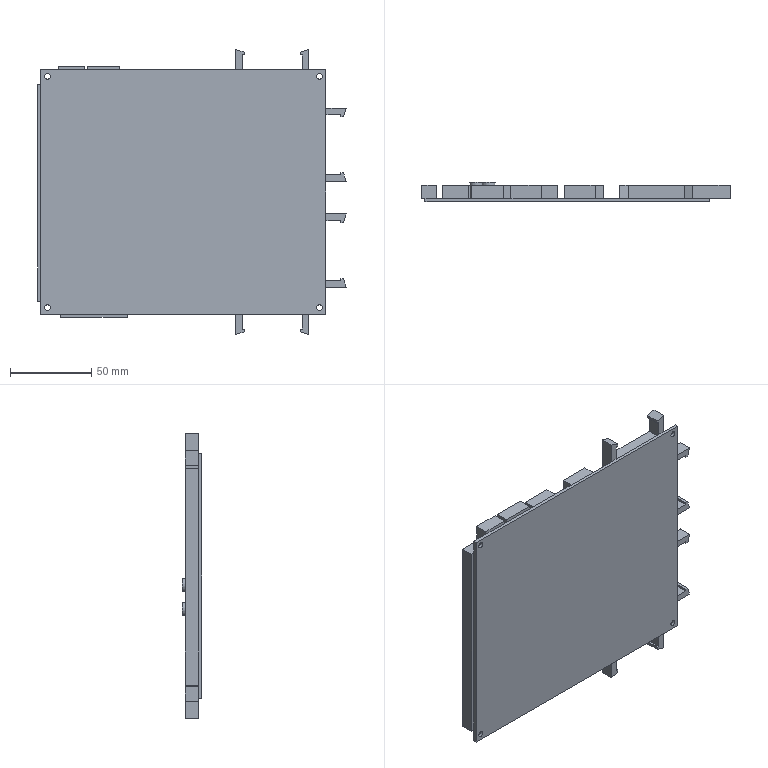Part | NX | features BREP 1 | 1 solid | 122 faces | box 189.5 x 12 x 175 mm | volume 96963 mm3 | plane 116 | cylinder 6 | commonest cylinder face diameters 3.5 x4 8 x2